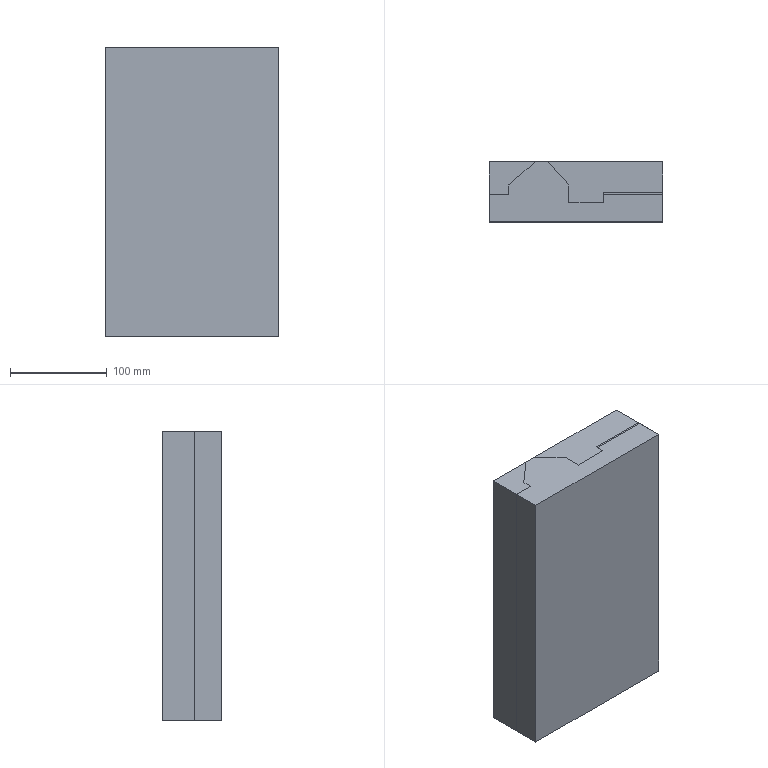NC program | NX | posted with a generic post | part box 180 x 62 x 300 mm
Lines 4322 to 5179 of 29776:
(型腔铣 , TOOL : D21R0.8圆鼻飞刀)
N8642 T04 M6
N8644 /M1
N8646 G54
N8648 G17 G0 G90 X-171.183 Y-112.918 S1500 M3
N8650 G43 Z20. H4
N8652 Z0.702
N8654 G94 G1 Z-0.298 F2000.
N8656 G2 X-156.411 Y-100.522 R15.
N8658 G1 X-151.484
N8660 G3 X-150.081 Y-100.542 R58.205
N8662 G1 X150.083
N8664 G3 X151.483 Y-100.522 R58.206
N8666 G1 X155.668
N8668 G3 X157.107 Y-100.065 R2.5 F1880.
N8670 X158.326 Y-99.083 R12.327 F1760.
N8672 X159.4 Y-97.966 R12.327 F1640.
N8674 X160.325 Y-96.724 R12.327 F1520.
N8676 X161.088 Y-95.375 R12.327 F1400.
N8678 X161.675 Y-93.941 R12.327 F1280.
N8680 X162.077 Y-92.445 R12.327 F1160.
N8682 X162.289 Y-90.91 R12.327 F1040.
N8684 X162.323 Y-89.996 R12.327 F920.
N8686 G1 Y-89.361
N8688 Y-87.81 F800.
N8690 G3 X159.825 Y-85.312 R2.5
N8692 G1 X151.268 F2000.
N8694 G2 X150.049 Y-85.332 R42.996
N8696 G1 X-150.048
N8698 G2 X-151.269 Y-85.312 R42.995
N8700 G1 X-159.824
N8702 G2 X-161.163 Y-84.923 R2.5 F1880.
N8704 X-162.085 Y-83.876 R2.5 F1760.
N8706 X-162.323 Y-82.813 R2.5 F1640.
N8708 G1 Y-82.497
N8710 Y-81.083 F1520.
N8712 Y-79.67 F1400.
N8714 Y-78.256 F1280.
N8716 Y-76.842 F1160.
N8718 Y-75.428 F1040.
N8720 Y-74.014 F920.
N8722 Y-72.6 F800.
N8724 G2 X-159.825 Y-70.102 R2.5
N8726 G1 X-151.011 F2000.
N8728 G3 X-150.028 Y-70.122 R27.785
N8730 G1 X150.028
N8732 G3 X151.01 Y-70.102 R27.786
N8734 G1 X160.275
N8736 G3 X161.59 Y-69.728 R2.5 F1880.
N8738 X162.512 Y-68.719 R2.5 F1760.
N8740 X162.726 Y-68.095 R2.5 F1640.
N8742 G1 X162.868 Y-67.386
N8744 X163.14 Y-66.029 F1520.
N8746 X163.413 Y-64.671 F1400.
N8748 X163.685 Y-63.314 F1280.
N8750 X163.957 Y-61.956 F1160.
N8752 X164.23 Y-60.599 F1040.
N8754 X164.502 Y-59.242 F920.
N8756 X164.774 Y-57.884 F800.
N8758 G3 X162.323 Y-54.892 R2.5
N8760 G1 X157.323
N8762 X152.323 F1040.
N8764 X150.664 F1280.
N8766 G2 X150. Y-54.912 R12.576
N8768 G1 X147.323
N8770 X142.323 F1520.
N8772 X137.323 F1760.
N8774 X-150. F2000.
N8776 G2 X-150.665 Y-54.892 R12.575
N8778 G1 X-162.323
N8780 G3 X-167.323 Y-56.232 R10.
N8782 G0 Z20.
N8784 X-170.885 Y-113.255
N8786 Z0.404
N8788 G1 Z-0.596
N8790 G2 X-156.113 Y-100.859 R15.
N8792 G1 X-151.49
N8794 G3 X-150.054 Y-100.879 R58.217
N8796 G1 X149.939
N8798 G3 X151.578 Y-100.859 R57.944
N8800 G1 X155.419
N8802 G3 X156.775 Y-100.458 R2.5 F1880.
N8804 G1 X156.889 Y-100.384
N8806 G3 X158.14 Y-99.436 R12.53 F1760.
N8808 X159.262 Y-98.339 R12.53 F1640.
N8810 X160.238 Y-97.111 R12.53 F1520.
N8812 X161.053 Y-95.771 R12.53 F1400.
N8814 G1 X161.083 Y-95.713 F1280.
N8816 X161.095 Y-95.69
N8818 G3 X161.684 Y-94.334 R12.846
N8820 X162.135 Y-92.831 R12.846 F1160.
N8822 X162.399 Y-91.285 R12.846 F1040.
N8824 X162.474 Y-90.01 R12.846 F920.
N8826 G1 Y-89.99
N8828 Y-89.718
N8830 Y-88.148 F800.
N8832 G3 X159.976 Y-85.649 R2.5
N8834 G1 X151.363 F2000.
N8836 G2 X149.955 Y-85.669 R42.734
N8838 G1 X-150.04
N8840 G2 X-151.275 Y-85.649 R43.007
N8842 G1 X-159.974
N8844 G2 X-161.314 Y-85.26 R2.5 F1880.
N8846 X-162.236 Y-84.213 R2.5 F1760.
N8848 X-162.474 Y-83.15 R2.5 F1640.
N8850 G1 Y-82.834
N8852 Y-81.42 F1520.
N8854 Y-80.007 F1400.
N8856 Y-78.593 F1280.
N8858 Y-77.179 F1160.
N8860 Y-75.765 F1040.
N8862 Y-74.351 F920.
N8864 Y-72.937 F800.
N8866 G2 X-159.976 Y-70.439 R2.5
N8868 G1 X-151.018 F2000.
N8870 G3 X-150.023 Y-70.459 R27.797
N8872 G1 X149.974
N8874 G3 X151.104 Y-70.439 R27.524
N8876 G1 X160.426
N8878 G3 X161.741 Y-70.066 R2.5 F1880.
N8880 X162.662 Y-69.056 R2.5 F1760.
N8882 X162.876 Y-68.432 R2.5 F1640.
N8884 G1 X163.019 Y-67.723
N8886 X163.291 Y-66.366 F1520.
N8888 X163.563 Y-65.008 F1400.
N8890 X163.836 Y-63.651 F1280.
N8892 X164.108 Y-62.294 F1160.
N8894 X164.38 Y-60.936 F1040.
N8896 X164.653 Y-59.579 F920.
N8898 X164.925 Y-58.221 F800.
N8900 G3 X162.474 Y-55.229 R2.5
N8902 G1 X157.474
N8904 X152.474 F1040.
N8906 X150.755 F1280.
N8908 G2 X150. Y-55.249 R12.314
N8910 G1 X147.474
N8912 X142.474 F1520.
N8914 X137.474 F1760.
N8916 X-150. F2000.
N8918 G2 X-150.672 Y-55.229 R12.587
N8920 G1 X-162.474
N8922 G3 X-167.474 Y-56.569 R10.
N8924 G0 Z20.
N8926 X-170.33 Y-113.592
N8928 Z0.105
N8930 G1 Z-0.895
N8932 G2 X-155.558 Y-101.197 R15.
N8934 G1 X-151.487
N8936 G3 X-150.099 Y-101.216 R58.228
N8938 G1 X150.035 Y-101.217
N8940 G3 X151.511 Y-101.197 R58.142
N8942 G1 X154.938
N8944 G3 X156.169 Y-100.872 R2.5 F1880.
N8946 X156.438 Y-100.715 R12.5
N8948 X157.752 Y-99.806 R12.5 F1760.
N8950 X158.939 Y-98.737 R12.5 F1640.
N8952 X159.981 Y-97.526 R12.5 F1520.
N8954 X160.859 Y-96.191 R12.5 F1400.
N8956 X161.56 Y-94.756 R12.5 F1280.
N8958 X162.072 Y-93.243 R12.5 F1160.
N8960 X162.387 Y-91.677 R12.5 F1040.
N8962 X162.5 Y-90.083 R12.5 F920.
N8964 G1 Y-90. F800.
N8966 Y-88.485
N8968 G3 X160.002 Y-85.987 R2.5
N8970 G1 X151.296 F2000.
N8972 G2 X150.022 Y-86.007 R42.932
N8974 G1 X-150.062
N8976 G2 X-151.272 Y-85.987 R43.018
N8978 G1 X-160.001
N8980 G2 X-161.34 Y-85.597 R2.5 F1880.
N8982 X-162.262 Y-84.55 R2.5 F1760.
N8984 X-162.5 Y-83.487 R2.5 F1640.
N8986 G1 Y-83.171
N8988 Y-81.758 F1520.
N8990 Y-80.344 F1400.
N8992 Y-78.93 F1280.
N8994 Y-77.516 F1160.
N8996 Y-76.102 F1040.
N8998 Y-74.688 F920.
N9000 Y-73.274 F800.
N9002 G2 X-160.002 Y-70.777 R2.5
N9004 G1 X-151.015 F2000.
N9006 G3 X-150.025 Y-70.797 R27.808
N9008 G1 X150.009
N9010 G3 X151.039 Y-70.777 R27.722
N9012 G1 X160.452
N9014 G3 X161.767 Y-70.403 R2.5 F1880.
N9016 X162.688 Y-69.393 R2.5 F1760.
N9018 X162.902 Y-68.769 R2.5 F1640.
N9020 G1 X163.045 Y-68.06
N9022 X163.317 Y-66.703 F1520.
N9024 X163.589 Y-65.346 F1400.
N9026 X163.862 Y-63.988 F1280.
N9028 X164.134 Y-62.631 F1160.
N9030 X164.406 Y-61.273 F1040.
N9032 X164.678 Y-59.916 F920.
N9034 X164.951 Y-58.558 F800.
N9036 G3 X162.5 Y-55.567 R2.5
N9038 G1 X157.5
N9040 X152.5 F1040.
N9042 X150.693 F1280.
N9044 G2 X150. Y-55.587 R12.512
N9046 G1 X147.5
N9048 X142.5 F1520.
N9050 X137.5 F1760.
N9052 X-150. F2000.
N9054 G2 X-150.669 Y-55.567 R12.598
N9056 G1 X-162.5
N9058 G3 X-167.5 Y-56.906 R10.
N9060 G0 Z20.
N9062 X-169.591 Y-113.929
N9064 Z-0.193
N9066 G1 Z-1.193
N9068 G2 X-154.819 Y-101.534 R15.
N9070 G1 X-151.49
N9072 G3 X-150.092 Y-101.554 R58.223
N9074 G1 X150.053
N9076 G3 X151.504 Y-101.534 R58.173
N9078 G1 X154.29
N9080 G3 X155.359 Y-101.293 R2.5 F1880.
N9082 X155.836 Y-101.054 R12.5
N9084 X157.23 Y-100.197 R12.5 F1760.
N9086 X158.501 Y-99.165 R12.5 F1640.
N9088 X159.625 Y-97.975 R12.5 F1520.
N9090 X160.585 Y-96.649 R12.5 F1400.
N9092 X161.363 Y-95.209 R12.5 F1280.
N9094 X161.946 Y-93.68 R12.5 F1160.
N9096 X162.324 Y-92.088 R12.5 F1040.
N9098 X162.492 Y-90.46 R12.5 F920.
N9100 X162.5 Y-90. R12.5 F800.
N9102 G1 Y-88.822
N9104 G3 X160.002 Y-86.324 R2.5
N9106 G1 X151.289 F2000.
N9108 G2 X150.034 Y-86.344 R42.963
N9110 G1 X-150.058
N9112 G2 X-151.275 Y-86.324 R43.013
N9114 G1 X-160.001
N9116 G2 X-161.34 Y-85.934 R2.5 F1880.
N9118 X-162.262 Y-84.887 R2.5 F1760.
N9120 X-162.5 Y-83.824 R2.5 F1640.
N9122 G1 Y-83.509
N9124 Y-82.095 F1520.
N9126 Y-80.681 F1400.
N9128 Y-79.267 F1280.
N9130 Y-77.853 F1160.
N9132 Y-76.439 F1040.
N9134 Y-75.026 F920.
N9136 Y-73.612 F800.
N9138 G2 X-160.002 Y-71.114 R2.5
N9140 G1 X-151.017 F2000.
N9142 G3 X-150.023 Y-71.134 R27.803
N9144 G1 X150.014
N9146 G3 X151.031 Y-71.114 R27.753
N9148 G1 X160.452
N9150 G3 X161.767 Y-70.74 R2.5 F1880.
N9152 X162.688 Y-69.73 R2.5 F1760.
N9154 X162.902 Y-69.106 R2.5 F1640.
N9156 G1 X163.045 Y-68.398
N9158 X163.317 Y-67.04 F1520.
N9160 X163.589 Y-65.683 F1400.
N9162 X163.862 Y-64.325 F1280.
N9164 X164.134 Y-62.968 F1160.
N9166 X164.406 Y-61.61 F1040.
N9168 X164.678 Y-60.253 F920.
N9170 X164.951 Y-58.895 F800.
N9172 G3 X162.5 Y-55.904 R2.5
N9174 G1 X157.5
N9176 X152.5 F1040.
N9178 X150.686 F1280.
N9180 G2 X150. Y-55.924 R12.543
N9182 G1 X147.5
N9184 X142.5 F1520.
N9186 X137.5 F1760.
N9188 X-150. F2000.
N9190 G2 X-150.672 Y-55.904 R12.593
N9192 G1 X-162.5
N9194 G3 X-167.5 Y-57.243 R10.
N9196 G0 Z20.
N9198 X-168.688 Y-114.266
N9200 Z-0.491
N9202 G1 Z-1.491
N9204 G2 X-153.916 Y-101.871 R15.
N9206 G1 X-151.457
N9208 G3 X-150.113 Y-101.891 R58.315
N9210 G1 X150.036
N9212 G3 X151.501 Y-101.871 R58.182
N9214 G1 X153.493
N9216 G3 X154.362 Y-101.714 R2.5 F1880.
N9218 X155.105 Y-101.41 R12.5
N9220 X156.597 Y-100.617 R12.5 F1760.
N9222 X157.969 Y-99.631 R12.5 F1640.
N9224 X159.195 Y-98.468 R12.5 F1520.
N9226 X160.253 Y-97.151 R12.5 F1400.
N9228 X161.123 Y-95.703 R12.5 F1280.
N9230 X161.791 Y-94.151 R12.5 F1160.
N9232 X162.243 Y-92.523 R12.5 F1040.
N9234 X162.471 Y-90.849 R12.5 F920.
N9236 X162.5 Y-90. R12.5 F800.
N9238 G1 Y-89.159
N9240 G3 X160.002 Y-86.661 R2.5
N9242 G1 X151.286 F2000.
N9244 G2 X150.027 Y-86.681 R42.972
N9246 G1 X-150.083
N9248 G2 X-151.241 Y-86.661 R43.105
N9250 G1 X-160.001
N9252 G2 X-161.34 Y-86.271 R2.5 F1880.
N9254 X-162.262 Y-85.225 R2.5 F1760.
N9256 X-162.5 Y-84.161 R2.5 F1640.
N9258 G1 Y-83.846
N9260 Y-82.432 F1520.
N9262 Y-81.018 F1400.
N9264 Y-79.604 F1280.
N9266 Y-78.19 F1160.
N9268 Y-76.777 F1040.
N9270 Y-75.363 F920.
N9272 Y-73.949 F800.
N9274 G2 X-160.002 Y-71.451 R2.5
N9276 G1 X-150.983 F2000.
N9278 G3 X-150.048 Y-71.471 R27.895
N9280 G1 X150.016
N9282 G3 X151.029 Y-71.451 R27.762
N9284 G1 X160.452
N9286 G3 X161.767 Y-71.077 R2.5 F1880.
N9288 X162.688 Y-70.067 R2.5 F1760.
N9290 X162.902 Y-69.443 R2.5 F1640.
N9292 G1 X163.045 Y-68.735
N9294 X163.317 Y-67.377 F1520.
N9296 X163.589 Y-66.02 F1400.
N9298 X163.862 Y-64.662 F1280.
N9300 X164.134 Y-63.305 F1160.
N9302 X164.406 Y-61.947 F1040.
N9304 X164.678 Y-60.59 F920.
N9306 X164.951 Y-59.233 F800.
N9308 G3 X162.5 Y-56.241 R2.5
N9310 G1 X157.5
N9312 X152.5 F1040.
N9314 X150.683 F1280.
N9316 G2 X150. Y-56.261 R12.552
N9318 G1 X147.5
N9320 X142.5 F1520.
N9322 X137.5 F1760.
N9324 X-150. F2000.
N9326 G2 X-150.636 Y-56.241 R12.685
N9328 G1 X-162.5
N9330 G3 X-167.5 Y-57.581 R10.
N9332 G0 Z20.
N9334 X-167.459 Y-114.603
N9336 Z-0.789
N9338 G1 Z-1.789
N9340 G2 X-152.686 Y-102.208 R15.
N9342 G1 X-151.487
N9344 G3 X-150.074 Y-102.228 R58.228
N9346 G1 X150.057
N9348 G3 X151.495 Y-102.208 R58.202
N9350 G1 X152.401
N9352 G3 X152.997 Y-102.135 R2.5 F1880.
N9354 X154.118 Y-101.802 R12.5
N9356 X155.743 Y-101.102 R12.5 F1760.
N9358 X157.254 Y-100.18 R12.5 F1640.
N9360 X158.619 Y-99.053 R12.5 F1520.
N9362 X159.811 Y-97.745 R12.5 F1400.
N9364 X160.807 Y-96.282 R12.5 F1280.
N9366 X161.586 Y-94.692 R12.5 F1160.
N9368 X162.132 Y-93.009 R12.5 F1040.
N9370 X162.436 Y-91.265 R12.5 F920.
N9372 X162.5 Y-90. R12.5 F800.
N9374 G1 Y-89.496
N9376 G3 X160.002 Y-86.998 R2.5
N9378 G1 X151.28 F2000.
N9380 G2 X150.034 Y-87.018 R42.992
N9382 G1 X-150.044
N9384 G2 X-151.272 Y-86.998 R43.019
N9386 G1 X-160.001
N9388 G2 X-161.34 Y-86.608 R2.5 F1880.
N9390 X-162.262 Y-85.562 R2.5 F1760.
N9392 X-162.5 Y-84.498 R2.5 F1640.
N9394 G1 Y-84.183
N9396 Y-82.769 F1520.
N9398 Y-81.355 F1400.
N9400 Y-79.941 F1280.
N9402 Y-78.527 F1160.
N9404 Y-77.114 F1040.
N9406 Y-75.7 F920.
N9408 Y-74.286 F800.
N9410 G2 X-160.002 Y-71.788 R2.5
N9412 G1 X-151.015 F2000.
N9414 G3 X-150.025 Y-71.808 R27.809
N9416 G1 X150.02
N9418 G3 X151.023 Y-71.788 R27.782
N9420 G1 X160.452
N9422 G3 X161.767 Y-71.414 R2.5 F1880.
N9424 X162.688 Y-70.404 R2.5 F1760.
N9426 X162.902 Y-69.78 R2.5 F1640.
N9428 G1 X163.045 Y-69.072
N9430 X163.317 Y-67.714 F1520.
N9432 X163.589 Y-66.357 F1400.
N9434 X163.862 Y-64.999 F1280.
N9436 X164.134 Y-63.642 F1160.
N9438 X164.406 Y-62.285 F1040.
N9440 X164.678 Y-60.927 F920.
N9442 X164.951 Y-59.57 F800.
N9444 G3 X162.5 Y-56.578 R2.5
N9446 G1 X157.5
N9448 X152.5 F1040.
N9450 X150.677 F1280.
N9452 G2 X150. Y-56.598 R12.572
N9454 G1 X147.5
N9456 X142.5 F1520.
N9458 X137.5 F1760.
N9460 X-150. F2000.
N9462 G2 X-150.669 Y-56.578 R12.599
N9464 G1 X-162.5
N9466 G3 X-167.5 Y-57.918 R10.
N9468 G0 Z20.
N9470 X-173.41 Y-111.43
N9472 Z-1.088
N9474 G1 Z-2.088
N9476 G2 X-158.638 Y-99.035 R15.
N9478 G1 X-151.443
N9480 G3 X-150.062 Y-99.055 R54.713
N9482 G1 X150.037
N9484 G3 X151.457 Y-99.035 R54.664
N9486 G1 X157.571
N9488 G3 X158.655 Y-98.787 R2.5 F1880.
N9490 X159.46 Y-98.17 R2.5 F1760.
N9492 G1 X159.525 Y-98.094
N9494 G3 X160.212 Y-97.208 R12.5 F1640.
N9496 X160.817 Y-96.264 R12.5 F1520.
N9498 X161.335 Y-95.27 R12.5 F1400.
N9500 X161.761 Y-94.233 R12.5 F1280.
N9502 X162.093 Y-93.163 R12.5 F1160.
N9504 X162.328 Y-92.066 R12.5 F1040.
N9506 X162.464 Y-90.954 R12.5 F920.
N9508 X162.5 Y-90. R12.5 F800.
N9510 G1 Y-89.833
N9512 G3 X160.002 Y-87.335 R2.5
N9514 G1 X151.289 F2000.
N9516 G2 X150.024 Y-87.355 R42.964
N9518 G1 X-150.041
N9520 G2 X-151.275 Y-87.335 R43.013
N9522 G1 X-160.
N9524 G2 X-161.34 Y-86.946 R2.5 F1880.
N9526 X-162.262 Y-85.899 R2.5 F1760.
N9528 X-162.5 Y-84.836 R2.5 F1640.
N9530 G1 Y-84.52
N9532 Y-83.106 F1520.
N9534 Y-81.692 F1400.
N9536 Y-80.278 F1280.
N9538 Y-78.865 F1160.
N9540 Y-77.451 F1040.
N9542 Y-76.037 F920.
N9544 Y-74.623 F800.
N9546 G2 X-160.002 Y-72.125 R2.5
N9548 G1 X-151.017 F2000.
N9550 G3 X-150.023 Y-72.145 R27.803
N9552 G1 X150.014
N9554 G3 X151.031 Y-72.125 R27.754
N9556 G1 X160.452
N9558 G3 X161.767 Y-71.751 R2.5 F1880.
N9560 X162.688 Y-70.742 R2.5 F1760.
N9562 X162.902 Y-70.117 R2.5 F1640.
N9564 G1 X163.045 Y-69.409
N9566 X163.317 Y-68.051 F1520.
N9568 X163.589 Y-66.694 F1400.
N9570 X163.862 Y-65.337 F1280.
N9572 X164.134 Y-63.979 F1160.
N9574 X164.406 Y-62.622 F1040.
N9576 X164.678 Y-61.264 F920.
N9578 X164.951 Y-59.907 F800.
N9580 G3 X162.5 Y-56.915 R2.5
N9582 G1 X157.5
N9584 X152.5 F1040.
N9586 X150.686 F1280.
N9588 G2 X150. Y-56.935 R12.544
N9590 G1 X147.5
N9592 X142.5 F1520.
N9594 X137.5 F1760.
N9596 X-150. F2000.
N9598 G2 X-150.672 Y-56.915 R12.593
N9600 G1 X-162.5
N9602 G3 X-167.5 Y-58.255 R10.
N9604 G0 Z20.
N9606 X-173.043 Y-111.767
N9608 Z-1.386
N9610 G1 Z-2.386
N9612 G2 X-158.271 Y-99.372 R15.
N9614 G1 X-151.41
N9616 G3 X-150.146 Y-99.392 R54.805
N9618 G1 X150.047
N9620 G3 X151.454 Y-99.372 R54.672
N9622 G1 X157.266
N9624 G3 X158.383 Y-99.108 R2.5 F1880.
N9626 X159.079 Y-98.592 R2.5 F1760.
N9628 X159.274 Y-98.381 R12.5
N9630 X160.01 Y-97.487 R12.5 F1640.
N9632 X160.66 Y-96.529 R12.5 F1520.
N9634 X161.218 Y-95.514 R12.5 F1400.
N9636 X161.68 Y-94.453 R12.5 F1280.
N9638 X162.042 Y-93.353 R12.5 F1160.
N9640 X162.3 Y-92.225 R12.5 F1040.
N9642 X162.454 Y-91.077 R12.5 F920.
N9644 X162.5 Y-90. R12.5 F800.
N9646 G1 Y-89.92
N9648 G3 X160.252 Y-87.672 R2.25
N9650 G1 X151.286 F2000.
N9652 G2 X150.038 Y-87.692 R42.972
N9654 G1 X-150.119
N9656 G2 X-151.241 Y-87.672 R43.105
N9658 G1 X-160.001
N9660 G2 X-161.34 Y-87.283 R2.5 F1880.
N9662 X-162.262 Y-86.236 R2.5 F1760.
N9664 X-162.5 Y-85.173 R2.5 F1640.
N9666 G1 Y-84.857
N9668 Y-83.443 F1520.
N9670 Y-82.029 F1400.
N9672 Y-80.616 F1280.
N9674 Y-79.202 F1160.
N9676 Y-77.788 F1040.
N9678 Y-76.374 F920.
N9680 Y-74.96 F800.
N9682 G2 X-160.002 Y-72.462 R2.5
N9684 G1 X-150.983 F2000.
N9686 G3 X-150.048 Y-72.482 R27.895
N9688 G1 X150.016
N9690 G3 X151.029 Y-72.462 R27.762
N9692 G1 X160.452
N9694 G3 X161.767 Y-72.088 R2.5 F1880.
N9696 X162.688 Y-71.079 R2.5 F1760.
N9698 X162.902 Y-70.454 R2.5 F1640.
N9700 G1 X163.045 Y-69.746
N9702 X163.317 Y-68.389 F1520.
N9704 X163.589 Y-67.031 F1400.
N9706 X163.862 Y-65.674 F1280.
N9708 X164.134 Y-64.316 F1160.
N9710 X164.406 Y-62.959 F1040.
N9712 X164.678 Y-61.601 F920.
N9714 X164.951 Y-60.244 F800.
N9716 G3 X162.5 Y-57.252 R2.5
N9718 G1 X157.5
N9720 X152.5 F1040.
N9722 X150.683 F1280.
N9724 G2 X150. Y-57.272 R12.552
N9726 G1 X147.5
N9728 X142.5 F1520.
N9730 X137.5 F1760.
N9732 X-150. F2000.
N9734 G2 X-150.636 Y-57.252 R12.685
N9736 G1 X-162.5
N9738 G3 X-167.5 Y-58.592 R10.
N9740 G0 Z20.
N9742 X-172.645 Y-112.105
N9744 Z-1.684
N9746 G1 Z-2.684
N9748 G2 X-157.873 Y-99.709 R15.
N9750 G1 X-151.44
N9752 G3 X-150.091 Y-99.729 R54.719
N9754 G1 X150.069
N9756 G3 X151.449 Y-99.709 R54.691
N9758 G1 X156.932
N9760 G3 X158.056 Y-99.441 R2.5 F1880.
N9762 X158.661 Y-99.013 R2.5 F1760.
N9764 X158.961 Y-98.715 R12.5
N9766 X159.734 Y-97.843 R12.5 F1640.
N9768 X160.422 Y-96.902 R12.5 F1520.
N9770 X161.02 Y-95.901 R12.5 F1400.
N9772 X161.521 Y-94.848 R12.5 F1280.
N9774 X161.923 Y-93.754 R12.5 F1160.
N9776 X162.221 Y-92.627 R12.5 F1040.
N9778 X162.412 Y-91.477 R12.5 F920.
N9780 X162.496 Y-90.314 R12.5 F800.
N9782 X160.249 Y-88.009 R2.25
N9784 G1 X151.281 F2000.
N9786 G2 X150.048 Y-88.029 R42.991
N9788 G1 X-150.062
N9790 G2 X-151.272 Y-88.009 R43.019
N9792 G1 X-160.001
N9794 G2 X-161.34 Y-87.62 R2.5 F1880.
N9796 X-162.262 Y-86.573 R2.5 F1760.
N9798 X-162.5 Y-85.51 R2.5 F1640.
N9800 G1 Y-85.194
N9802 Y-83.78 F1520.
N9804 Y-82.366 F1400.
N9806 Y-80.953 F1280.
N9808 Y-79.539 F1160.
N9810 Y-78.125 F1040.
N9812 Y-76.711 F920.
N9814 Y-75.297 F800.
N9816 G2 X-160.002 Y-72.799 R2.5
N9818 G1 X-151.014 F2000.
N9820 G3 X-150.025 Y-72.819 R27.809
N9822 G1 X150.019
N9824 G3 X151.023 Y-72.799 R27.781
N9826 G1 X160.452
N9828 G3 X161.767 Y-72.425 R2.5 F1880.
N9830 X162.688 Y-71.416 R2.5 F1760.
N9832 X162.902 Y-70.792 R2.5 F1640.
N9834 G1 X163.045 Y-70.083
N9836 X163.317 Y-68.726 F1520.
N9838 X163.589 Y-67.368 F1400.
N9840 X163.862 Y-66.011 F1280.
N9842 X164.134 Y-64.653 F1160.
N9844 X164.406 Y-63.296 F1040.
N9846 X164.678 Y-61.938 F920.
N9848 X164.951 Y-60.581 F800.
N9850 G3 X162.5 Y-57.589 R2.5
N9852 G1 X157.5
N9854 X152.5 F1040.
N9856 X150.678 F1280.
N9858 G2 X150. Y-57.609 R12.571
N9860 G1 X147.5
N9862 X142.5 F1520.
N9864 X137.5 F1760.
N9866 X-150. F2000.
N9868 G2 X-150.669 Y-57.589 R12.599
N9870 G1 X-162.5
N9872 G3 X-167.5 Y-58.929 R10.
N9874 G0 Z20.
N9876 X-172.21 Y-112.442
N9878 Z-1.982
N9880 G1 Z-2.982
N9882 G2 X-157.438 Y-100.046 R15.
N9884 G1 X-151.443
N9886 G3 X-150.062 Y-100.066 R54.713
N9888 G1 X150.037
N9890 G3 X151.456 Y-100.046 R54.665
N9892 G1 X156.563
N9894 G3 X157.695 Y-99.774 R2.5 F1880.
N9896 X158.2 Y-99.434 R2.5 F1760.
N9898 X158.618 Y-99.054 R12.5
N9900 X159.43 Y-98.205 R12.5 F1640.
N9902 X160.158 Y-97.284 R12.5 F1520.
N9904 X160.797 Y-96.298 R12.5 F1400.
N9906 X161.341 Y-95.257 R12.5 F1280.
N9908 X161.784 Y-94.169 R12.5 F1160.
N9910 X162.124 Y-93.045 R12.5 F1040.
N9912 X162.356 Y-91.893 R12.5 F920.
N9914 X162.479 Y-90.725 R12.5 F800.
N9916 X160.234 Y-88.346 R2.25
N9918 G1 X151.288 F2000.
N9920 G2 X150.024 Y-88.366 R42.965
N9922 G1 X-150.041
N9924 G2 X-151.275 Y-88.346 R43.013
N9926 G1 X-160.001
N9928 G2 X-161.34 Y-87.957 R2.5 F1880.
N9930 X-162.262 Y-86.91 R2.5 F1760.
N9932 X-162.5 Y-85.847 R2.5 F1640.
N9934 G1 Y-85.531
N9936 Y-84.117 F1520.
N9938 Y-82.704 F1400.
N9940 Y-81.29 F1280.
N9942 Y-79.876 F1160.
N9944 Y-78.462 F1040.
N9946 Y-77.048 F920.
N9948 Y-75.634 F800.
N9950 G2 X-160.002 Y-73.136 R2.5
N9952 G1 X-151.017 F2000.
N9954 G3 X-150.023 Y-73.156 R27.803
N9956 G1 X150.014
N9958 G3 X151.031 Y-73.136 R27.755
N9960 G1 X160.452
N9962 G3 X161.767 Y-72.762 R2.5 F1880.
N9964 X162.688 Y-71.753 R2.5 F1760.
N9966 X162.902 Y-71.129 R2.5 F1640.
N9968 G1 X163.045 Y-70.42
N9970 X163.317 Y-69.063 F1520.
N9972 X163.589 Y-67.705 F1400.
N9974 X163.862 Y-66.348 F1280.
N9976 X164.134 Y-64.99 F1160.
N9978 X164.406 Y-63.633 F1040.
N9980 X164.678 Y-62.276 F920.
N9982 X164.951 Y-60.918 F800.
N9984 G3 X162.5 Y-57.926 R2.5
N9986 G1 X157.5
N9988 X152.5 F1040.
N9990 X150.685 F1280.
N9992 G2 X150. Y-57.946 R12.545
N9994 G1 X147.5
N9996 X142.5 F1520.
N9998 X137.5 F1760.
N10000 X-150. F2000.
N10002 G2 X-150.672 Y-57.926 R12.593
N10004 G1 X-162.5
N10006 G3 X-167.5 Y-59.266 R10.
N10008 G0 Z20.
N10010 X-171.732 Y-112.779
N10012 Z-2.281
N10014 G1 Z-3.281
N10016 G2 X-156.959 Y-100.383 R15.
N10018 G1 X-151.41
N10020 G3 X-150.146 Y-100.403 R54.805
N10022 G1 X150.047
N10024 G3 X151.454 Y-100.383 R54.672
N10026 G1 X156.154
N10028 G3 X157.297 Y-100.106 R2.5 F1880.
N10030 X157.689 Y-99.856 R2.5 F1760.
N10032 X158.244 Y-99.396 R12.5
N10034 X159.098 Y-98.572 R12.5 F1640.
N10036 X159.869 Y-97.671 R12.5 F1520.
N10038 X160.552 Y-96.701 R12.5 F1400.
N10040 X161.14 Y-95.67 R12.5 F1280.
N10042 X161.627 Y-94.589 R12.5 F1160.
N10044 X162.01 Y-93.466 R12.5 F1040.
N10046 X162.284 Y-92.311 R12.5 F920.
N10048 X162.448 Y-91.136 R12.5 F800.
N10050 X160.209 Y-88.683 R2.25
N10052 G1 X151.286 F2000.
N10054 G2 X150.038 Y-88.703 R42.972
N10056 G1 X-150.119
N10058 G2 X-151.241 Y-88.683 R43.105
N10060 G1 X-160.001
N10062 G2 X-161.34 Y-88.294 R2.5 F1880.
N10064 X-162.262 Y-87.247 R2.5 F1760.
N10066 X-162.5 Y-86.184 R2.5 F1640.
N10068 G1 Y-85.868
N10070 Y-84.455 F1520.
N10072 Y-83.041 F1400.
N10074 Y-81.627 F1280.
N10076 Y-80.213 F1160.
N10078 Y-78.799 F1040.
N10080 Y-77.385 F920.
N10082 Y-75.972 F800.
N10084 G2 X-160.002 Y-73.473 R2.5
N10086 G1 X-150.983 F2000.
N10088 G3 X-150.048 Y-73.493 R27.895
N10090 G1 X150.016
N10092 G3 X151.029 Y-73.473 R27.762
N10094 G1 X160.452
N10096 G3 X161.767 Y-73.1 R2.5 F1880.
N10098 X162.688 Y-72.09 R2.5 F1760.
N10100 X162.902 Y-71.466 R2.5 F1640.
N10102 G1 X163.045 Y-70.757
N10104 X163.317 Y-69.4 F1520.
N10106 X163.589 Y-68.042 F1400.
N10108 X163.862 Y-66.685 F1280.
N10110 X164.134 Y-65.328 F1160.
N10112 X164.406 Y-63.97 F1040.
N10114 X164.678 Y-62.613 F920.
N10116 X164.951 Y-61.255 F800.
N10118 G3 X162.5 Y-58.263 R2.5
N10120 G1 X157.5
N10122 X152.5 F1040.
N10124 X150.683 F1280.
N10126 G2 X150. Y-58.283 R12.552
N10128 G1 X147.5
N10130 X142.5 F1520.
N10132 X137.5 F1760.
N10134 X-150. F2000.
N10136 G2 X-150.636 Y-58.263 R12.685
N10138 G1 X-162.5
N10140 G3 X-167.5 Y-59.603 R10.
N10142 G0 Z20.
N10144 X-171.2 Y-113.116
N10146 Z-2.579
N10148 G1 Z-3.579
N10150 G2 X-156.428 Y-100.721 R15.
N10152 G1 X-151.44
N10154 G3 X-150.091 Y-100.741 R54.719
N10156 G1 X150.069
N10158 G3 X151.449 Y-100.721 R54.69
N10160 G1 X155.696
N10162 G3 X156.882 Y-100.42 R2.5 F1880.
N10164 X157.116 Y-100.277 R2.5 F1760.
N10166 X157.885 Y-99.7 R12.5
N10168 X158.804 Y-98.874 R12.5 F1640.
N10170 X159.637 Y-97.961 R12.5 F1520.
N10172 X160.376 Y-96.971 R12.5 F1400.
N10174 X161.013 Y-95.913 R12.5 F1280.
N10176 X161.543 Y-94.797 R12.5 F1160.
N10178 X161.96 Y-93.634 R12.5 F1040.
N10180 X162.26 Y-92.435 R12.5 F920.
N10182 X162.441 Y-91.213 R12.5 F800.
N10184 X160.452 Y-89.021 R2.
N10186 G1 X151.281 F2000.
N10188 G2 X150.047 Y-89.041 R42.99
N10190 G1 X-150.062
N10192 G2 X-151.272 Y-89.021 R43.019
N10194 G1 X-160.001
N10196 G2 X-161.34 Y-88.631 R2.5 F1880.
N10198 X-162.262 Y-87.584 R2.5 F1760.
N10200 X-162.5 Y-86.521 R2.5 F1640.
N10202 G1 Y-86.206
N10204 Y-84.792 F1520.
N10206 Y-83.378 F1400.
N10208 Y-81.964 F1280.
N10210 Y-80.55 F1160.
N10212 Y-79.136 F1040.
N10214 Y-77.722 F920.
N10216 Y-76.309 F800.
N10218 G2 X-160.002 Y-73.811 R2.5
N10220 G1 X-151.014 F2000.
N10222 G3 X-150.025 Y-73.831 R27.809
N10224 G1 X150.019
N10226 G3 X151.023 Y-73.811 R27.78
N10228 G1 X160.452
N10230 G3 X161.767 Y-73.437 R2.5 F1880.
N10232 X162.688 Y-72.427 R2.5 F1760.
N10234 X162.902 Y-71.803 R2.5 F1640.
N10236 G1 X163.045 Y-71.094
N10238 X163.317 Y-69.737 F1520.
N10240 X163.589 Y-68.38 F1400.
N10242 X163.862 Y-67.022 F1280.
N10244 X164.134 Y-65.665 F1160.
N10246 X164.406 Y-64.307 F1040.
N10248 X164.678 Y-62.95 F920.
N10250 X164.951 Y-61.592 F800.
N10252 G3 X162.5 Y-58.601 R2.5
N10254 G1 X157.5
N10256 X152.5 F1040.
N10258 X150.678 F1280.
N10260 G2 X150. Y-58.621 R12.57
N10262 G1 X147.5
N10264 X142.5 F1520.
N10266 X137.5 F1760.
N10268 X-150. F2000.
N10270 G2 X-150.669 Y-58.601 R12.599
N10272 G1 X-162.5
N10274 G3 X-167.5 Y-59.94 R10.
N10276 G0 Z20.
N10278 X-170.601 Y-113.453
N10280 Z-2.877
N10282 G1 Z-3.877
N10284 G2 X-155.829 Y-101.058 R15.
N10286 G1 X-151.443
N10288 G3 X-150.084 Y-101.078 R54.713
N10290 G1 X150.05
N10292 G3 X151.456 Y-101.058 R54.666
N10294 G1 X155.175
N10296 G3 X156.38 Y-100.747 R2.5 F1880.
N10298 G1 X156.465 Y-100.698 F1760.
N10300 G3 X157.429 Y-100.053 R12.5
N10302 X158.401 Y-99.256 R12.5 F1640.
N10304 X159.288 Y-98.366 R12.5 F1520.
N10306 X160.081 Y-97.39 R12.5 F1400.
N10308 X160.773 Y-96.34 R12.5 F1280.
N10310 X161.355 Y-95.226 R12.5 F1160.
N10312 X161.823 Y-94.059 R12.5 F1040.
N10314 X162.17 Y-92.851 R12.5 F920.
N10316 X162.395 Y-91.614 R12.5 F800.
N10318 X160.414 Y-89.358 R2.
N10320 G1 X151.288 F2000.
N10322 G2 X150.034 Y-89.378 R42.966
N10324 G1 X-150.058
N10326 G2 X-151.275 Y-89.358 R43.013
N10328 G1 X-160.001
N10330 G2 X-161.34 Y-88.968 R2.5 F1880.
N10332 X-162.262 Y-87.921 R2.5 F1760.
N10334 X-162.5 Y-86.858 R2.5 F1640.
N10336 G1 Y-86.543
N10338 Y-85.129 F1520.
N10340 Y-83.715 F1400.
N10342 Y-82.301 F1280.
N10344 Y-80.887 F1160.
N10346 Y-79.473 F1040.
N10348 Y-78.06 F920.
N10350 Y-76.646 F800.